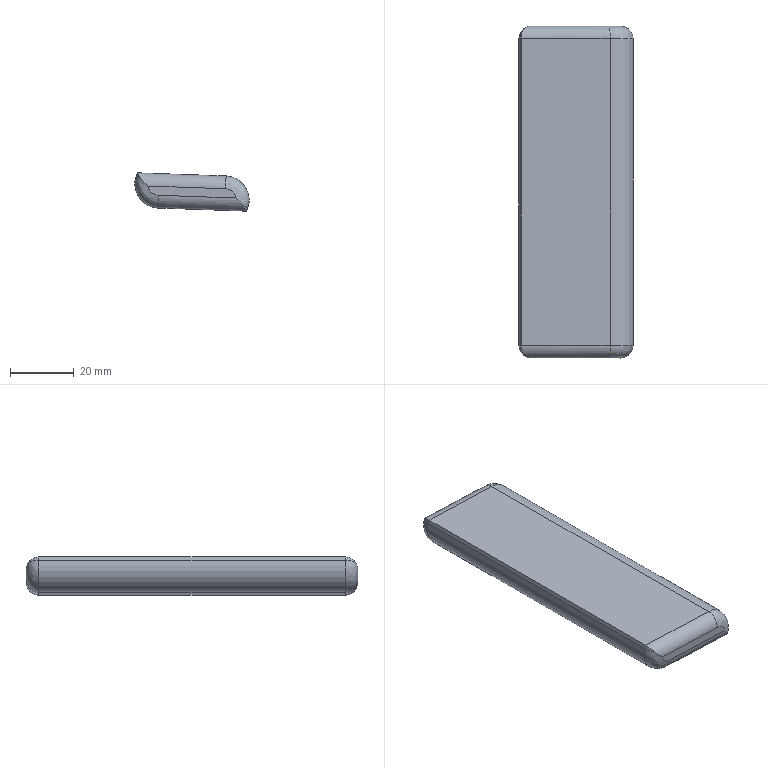Part | STEP file | solid 28 | 1 solid | 20 faces | box 35.828 x 104 x 11.998 mm | volume 37179 mm3 | cylinder 10 | plane 6 | spline 4 | commonest cylinder face diameters 8 x8 15 x2